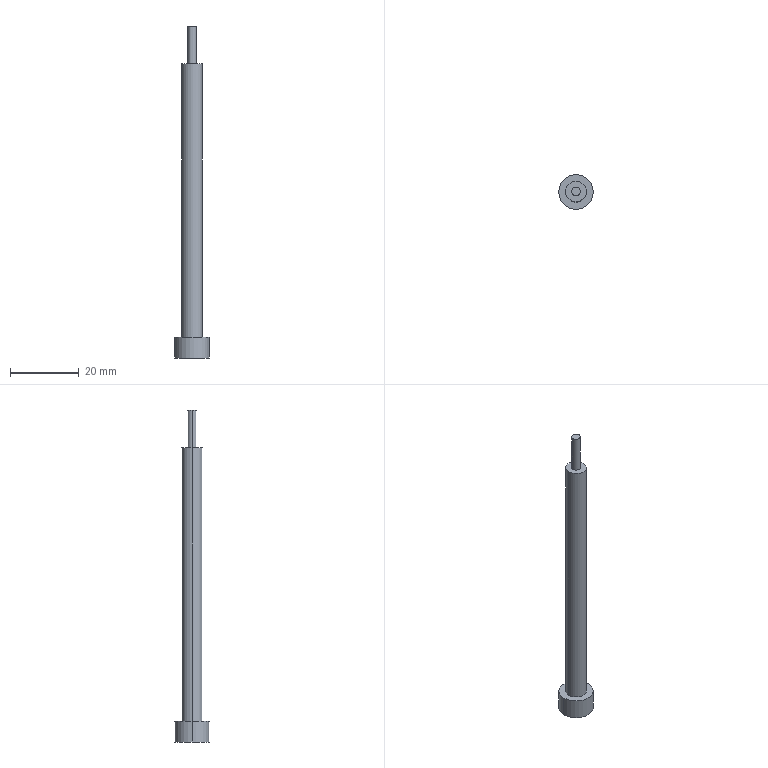Part | Creo | 1 solid | 10 faces | box 10 x 10 x 96.628 mm | volume 2777 mm3 | cylinder 6 | plane 4 | commonest cylinder face diameters 2.5 x2 6 x2 10 x2
STEP:
#1=CARTESIAN_POINT('',(-84.,-40.5,-87.5));
#2=VERTEX_POINT('',#1);
#3=CARTESIAN_POINT('',(-94.,-40.5,-87.5));
#4=VERTEX_POINT('',#3);
#5=CARTESIAN_POINT('',(-89.,-40.5,-87.5));
#6=DIRECTION('',(0.,0.,1.));
#7=DIRECTION('',(1.,0.,0.));
#8=AXIS2_PLACEMENT_3D('',#5,#6,#7);
#9=CIRCLE('',#8,5.);
#10=EDGE_CURVE('',#2,#4,#9,.T.);
#11=ORIENTED_EDGE('',*,*,#10,.F.);
#12=CARTESIAN_POINT('',(-89.,-40.5,-87.5));
#13=DIRECTION('',(0.,0.,1.));
#14=DIRECTION('',(-1.,0.,0.));
#15=AXIS2_PLACEMENT_3D('',#12,#13,#14);
#16=CIRCLE('',#15,5.);
#17=EDGE_CURVE('',#4,#2,#16,.T.);
#18=ORIENTED_EDGE('',*,*,#17,.F.);
#19=EDGE_LOOP('',(#11,#18));
#20=FACE_OUTER_BOUND('',#19,.F.);
#21=CARTESIAN_POINT('',(-86.,-40.5,-87.5));
#22=VERTEX_POINT('',#21);
#23=CARTESIAN_POINT('',(-92.,-40.5,-87.5));
#24=VERTEX_POINT('',#23);
#25=CARTESIAN_POINT('',(-89.,-40.5,-87.5));
#26=DIRECTION('',(0.,0.,-1.));
#27=DIRECTION('',(1.,0.,0.));
#28=AXIS2_PLACEMENT_3D('',#25,#26,#27);
#29=CIRCLE('',#28,3.);
#30=EDGE_CURVE('',#22,#24,#29,.T.);
#31=ORIENTED_EDGE('',*,*,#30,.F.);
#32=CARTESIAN_POINT('',(-89.,-40.5,-87.5));
#33=DIRECTION('',(0.,0.,-1.));
#34=DIRECTION('',(-1.,0.,0.));
#35=AXIS2_PLACEMENT_3D('',#32,#33,#34);
#36=CIRCLE('',#35,3.);
#37=EDGE_CURVE('',#24,#22,#36,.T.);
#38=ORIENTED_EDGE('',*,*,#37,.F.);
#39=EDGE_LOOP('',(#31,#38));
#40=FACE_BOUND('',#39,.F.);
#41=CARTESIAN_POINT('',(-89.,-40.5,-87.5));
#42=DIRECTION('',(0.,0.,1.));
#43=DIRECTION('',(1.,0.,0.));
#44=AXIS2_PLACEMENT_3D('',#41,#42,#43);
#45=PLANE('',#44);
#46=ADVANCED_FACE('',(#20,#40),#45,.T.);
#47=CARTESIAN_POINT('',(-92.,-40.5,-7.872));
#48=VERTEX_POINT('',#47);
#49=CARTESIAN_POINT('',(-86.,-40.5,-7.872));
#50=VERTEX_POINT('',#49);
#51=CARTESIAN_POINT('',(-89.,-40.5,-7.872));
#52=DIRECTION('',(0.,0.,1.));
#53=DIRECTION('',(-1.,0.,0.));
#54=AXIS2_PLACEMENT_3D('',#51,#52,#53);
#55=CIRCLE('',#54,3.);
#56=EDGE_CURVE('',#48,#50,#55,.T.);
#57=ORIENTED_EDGE('',*,*,#56,.T.);
#58=CARTESIAN_POINT('',(-86.,-40.5,-87.5));
#59=DIRECTION('',(0.,0.,1.));
#60=VECTOR('',#59,79.628);
#61=LINE('',#58,#60);
#62=EDGE_CURVE('',#22,#50,#61,.T.);
#63=ORIENTED_EDGE('',*,*,#62,.F.);
#64=ORIENTED_EDGE('',*,*,#30,.T.);
#65=CARTESIAN_POINT('',(-92.,-40.5,-87.5));
#66=DIRECTION('',(0.,0.,1.));
#67=VECTOR('',#66,79.628);
#68=LINE('',#65,#67);
#69=EDGE_CURVE('',#24,#48,#68,.T.);
#70=ORIENTED_EDGE('',*,*,#69,.T.);
#71=EDGE_LOOP('',(#57,#63,#64,#70));
#72=FACE_OUTER_BOUND('',#71,.F.);
#73=CARTESIAN_POINT('',(-89.,-40.5,-87.5));
#74=DIRECTION('',(0.,0.,1.));
#75=DIRECTION('',(1.,0.,0.));
#76=AXIS2_PLACEMENT_3D('',#73,#74,#75);
#77=CYLINDRICAL_SURFACE('',#76,3.);
#78=ADVANCED_FACE('',(#72),#77,.T.);
#79=ORIENTED_EDGE('',*,*,#56,.F.);
#80=CARTESIAN_POINT('',(-89.,-40.5,-7.872));
#81=DIRECTION('',(0.,0.,1.));
#82=DIRECTION('',(1.,0.,0.));
#83=AXIS2_PLACEMENT_3D('',#80,#81,#82);
#84=CIRCLE('',#83,3.);
#85=EDGE_CURVE('',#50,#48,#84,.T.);
#86=ORIENTED_EDGE('',*,*,#85,.F.);
#87=EDGE_LOOP('',(#79,#86));
#88=FACE_OUTER_BOUND('',#87,.F.);
#89=CARTESIAN_POINT('',(-90.25,-40.5,-7.872));
#90=VERTEX_POINT('',#89);
#91=CARTESIAN_POINT('',(-87.75,-40.5,-7.872));
#92=VERTEX_POINT('',#91);
#93=CARTESIAN_POINT('',(-89.,-40.5,-7.872));
#94=DIRECTION('',(0.,0.,-1.));
#95=DIRECTION('',(-1.,0.,0.));
#96=AXIS2_PLACEMENT_3D('',#93,#94,#95);
#97=CIRCLE('',#96,1.25);
#98=EDGE_CURVE('',#90,#92,#97,.T.);
#99=ORIENTED_EDGE('',*,*,#98,.F.);
#100=CARTESIAN_POINT('',(-89.,-40.5,-7.872));
#101=DIRECTION('',(0.,0.,-1.));
#102=DIRECTION('',(1.,0.,0.));
#103=AXIS2_PLACEMENT_3D('',#100,#101,#102);
#104=CIRCLE('',#103,1.25);
#105=EDGE_CURVE('',#92,#90,#104,.T.);
#106=ORIENTED_EDGE('',*,*,#105,.F.);
#107=EDGE_LOOP('',(#99,#106));
#108=FACE_BOUND('',#107,.F.);
#109=CARTESIAN_POINT('',(-89.,-40.5,-7.872));
#110=DIRECTION('',(0.,0.,-1.));
#111=DIRECTION('',(0.,1.,0.));
#112=AXIS2_PLACEMENT_3D('',#109,#110,#111);
#113=PLANE('',#112);
#114=ADVANCED_FACE('',(#88,#108),#113,.F.);
#115=CARTESIAN_POINT('',(-87.75,-40.5,3.128));
#116=VERTEX_POINT('',#115);
#117=CARTESIAN_POINT('',(-90.25,-40.5,3.128));
#118=VERTEX_POINT('',#117);
#119=CARTESIAN_POINT('',(-89.,-40.5,3.128));
#120=DIRECTION('',(0.,0.,1.));
#121=DIRECTION('',(1.,0.,0.));
#122=AXIS2_PLACEMENT_3D('',#119,#120,#121);
#123=CIRCLE('',#122,1.25);
#124=EDGE_CURVE('',#116,#118,#123,.T.);
#125=ORIENTED_EDGE('',*,*,#124,.T.);
#126=CARTESIAN_POINT('',(-90.25,-40.5,-7.872));
#127=DIRECTION('',(0.,0.,1.));
#128=VECTOR('',#127,11.);
#129=LINE('',#126,#128);
#130=EDGE_CURVE('',#90,#118,#129,.T.);
#131=ORIENTED_EDGE('',*,*,#130,.F.);
#132=ORIENTED_EDGE('',*,*,#98,.T.);
#133=CARTESIAN_POINT('',(-87.75,-40.5,-7.872));
#134=DIRECTION('',(0.,0.,1.));
#135=VECTOR('',#134,11.);
#136=LINE('',#133,#135);
#137=EDGE_CURVE('',#92,#116,#136,.T.);
#138=ORIENTED_EDGE('',*,*,#137,.T.);
#139=EDGE_LOOP('',(#125,#131,#132,#138));
#140=FACE_OUTER_BOUND('',#139,.F.);
#141=CARTESIAN_POINT('',(-89.,-40.5,-6.872));
#142=DIRECTION('',(0.,0.,1.));
#143=DIRECTION('',(1.,0.,0.));
#144=AXIS2_PLACEMENT_3D('',#141,#142,#143);
#145=CYLINDRICAL_SURFACE('',#144,1.25);
#146=ADVANCED_FACE('',(#140),#145,.T.);
#147=ORIENTED_EDGE('',*,*,#124,.F.);
#148=CARTESIAN_POINT('',(-89.,-40.5,3.128));
#149=DIRECTION('',(0.,0.,1.));
#150=DIRECTION('',(-1.,0.,0.));
#151=AXIS2_PLACEMENT_3D('',#148,#149,#150);
#152=CIRCLE('',#151,1.25);
#153=EDGE_CURVE('',#118,#116,#152,.T.);
#154=ORIENTED_EDGE('',*,*,#153,.F.);
#155=EDGE_LOOP('',(#147,#154));
#156=FACE_OUTER_BOUND('',#155,.F.);
#157=CARTESIAN_POINT('',(0.,0.,3.128));
#158=DIRECTION('',(0.,0.,1.));
#159=DIRECTION('',(0.,1.,0.));
#160=AXIS2_PLACEMENT_3D('',#157,#158,#159);
#161=PLANE('',#160);
#162=ADVANCED_FACE('',(#156),#161,.T.);
#163=ORIENTED_EDGE('',*,*,#153,.T.);
#164=ORIENTED_EDGE('',*,*,#137,.F.);
#165=ORIENTED_EDGE('',*,*,#105,.T.);
#166=ORIENTED_EDGE('',*,*,#130,.T.);
#167=EDGE_LOOP('',(#163,#164,#165,#166));
#168=FACE_OUTER_BOUND('',#167,.F.);
#169=CARTESIAN_POINT('',(-89.,-40.5,-6.872));
#170=DIRECTION('',(0.,0.,1.));
#171=DIRECTION('',(1.,0.,0.));
#172=AXIS2_PLACEMENT_3D('',#169,#170,#171);
#173=CYLINDRICAL_SURFACE('',#172,1.25);
#174=ADVANCED_FACE('',(#168),#173,.T.);
#175=ORIENTED_EDGE('',*,*,#85,.T.);
#176=ORIENTED_EDGE('',*,*,#69,.F.);
#177=ORIENTED_EDGE('',*,*,#37,.T.);
#178=ORIENTED_EDGE('',*,*,#62,.T.);
#179=EDGE_LOOP('',(#175,#176,#177,#178));
#180=FACE_OUTER_BOUND('',#179,.F.);
#181=CARTESIAN_POINT('',(-89.,-40.5,-87.5));
#182=DIRECTION('',(0.,0.,1.));
#183=DIRECTION('',(1.,0.,0.));
#184=AXIS2_PLACEMENT_3D('',#181,#182,#183);
#185=CYLINDRICAL_SURFACE('',#184,3.);
#186=ADVANCED_FACE('',(#180),#185,.T.);
#187=ORIENTED_EDGE('',*,*,#10,.T.);
#188=CARTESIAN_POINT('',(-94.,-40.5,-93.5));
#189=VERTEX_POINT('',#188);
#190=CARTESIAN_POINT('',(-94.,-40.5,-93.5));
#191=DIRECTION('',(0.,0.,1.));
#192=VECTOR('',#191,6.);
#193=LINE('',#190,#192);
#194=EDGE_CURVE('',#189,#4,#193,.T.);
#195=ORIENTED_EDGE('',*,*,#194,.F.);
#196=CARTESIAN_POINT('',(-84.,-40.5,-93.5));
#197=VERTEX_POINT('',#196);
#198=CARTESIAN_POINT('',(-89.,-40.5,-93.5));
#199=DIRECTION('',(0.,0.,-1.));
#200=DIRECTION('',(-1.,0.,0.));
#201=AXIS2_PLACEMENT_3D('',#198,#199,#200);
#202=CIRCLE('',#201,5.);
#203=EDGE_CURVE('',#189,#197,#202,.T.);
#204=ORIENTED_EDGE('',*,*,#203,.T.);
#205=CARTESIAN_POINT('',(-84.,-40.5,-93.5));
#206=DIRECTION('',(0.,0.,1.));
#207=VECTOR('',#206,6.);
#208=LINE('',#205,#207);
#209=EDGE_CURVE('',#197,#2,#208,.T.);
#210=ORIENTED_EDGE('',*,*,#209,.T.);
#211=EDGE_LOOP('',(#187,#195,#204,#210));
#212=FACE_OUTER_BOUND('',#211,.F.);
#213=CARTESIAN_POINT('',(-89.,-40.5,-93.5));
#214=DIRECTION('',(0.,0.,1.));
#215=DIRECTION('',(1.,0.,0.));
#216=AXIS2_PLACEMENT_3D('',#213,#214,#215);
#217=CYLINDRICAL_SURFACE('',#216,5.);
#218=ADVANCED_FACE('',(#212),#217,.T.);
#219=ORIENTED_EDGE('',*,*,#17,.T.);
#220=ORIENTED_EDGE('',*,*,#209,.F.);
#221=CARTESIAN_POINT('',(-89.,-40.5,-93.5));
#222=DIRECTION('',(0.,0.,-1.));
#223=DIRECTION('',(1.,0.,0.));
#224=AXIS2_PLACEMENT_3D('',#221,#222,#223);
#225=CIRCLE('',#224,5.);
#226=EDGE_CURVE('',#197,#189,#225,.T.);
#227=ORIENTED_EDGE('',*,*,#226,.T.);
#228=ORIENTED_EDGE('',*,*,#194,.T.);
#229=EDGE_LOOP('',(#219,#220,#227,#228));
#230=FACE_OUTER_BOUND('',#229,.F.);
#231=CARTESIAN_POINT('',(-89.,-40.5,-93.5));
#232=DIRECTION('',(0.,0.,1.));
#233=DIRECTION('',(1.,0.,0.));
#234=AXIS2_PLACEMENT_3D('',#231,#232,#233);
#235=CYLINDRICAL_SURFACE('',#234,5.);
#236=ADVANCED_FACE('',(#230),#235,.T.);
#237=ORIENTED_EDGE('',*,*,#203,.F.);
#238=ORIENTED_EDGE('',*,*,#226,.F.);
#239=EDGE_LOOP('',(#237,#238));
#240=FACE_OUTER_BOUND('',#239,.F.);
#241=CARTESIAN_POINT('',(-89.,-40.5,-93.5));
#242=DIRECTION('',(0.,0.,-1.));
#243=DIRECTION('',(-1.,0.,0.));
#244=AXIS2_PLACEMENT_3D('',#241,#242,#243);
#245=PLANE('',#244);
#246=ADVANCED_FACE('',(#240),#245,.T.);
#247=CLOSED_SHELL('',(#46,#78,#114,#146,#162,#174,#186,#218,#236,#246));
#248=MANIFOLD_SOLID_BREP('',#247);
#249=(LENGTH_UNIT()NAMED_UNIT(*)SI_UNIT(.MILLI.,.METRE.));
#250=UNCERTAINTY_MEASURE_WITH_UNIT(LENGTH_MEASURE(0.009765),#249,'','');
#251=(NAMED_UNIT(*)PLANE_ANGLE_UNIT()SI_UNIT($,.RADIAN.));
#252=PLANE_ANGLE_MEASURE_WITH_UNIT(PLANE_ANGLE_MEASURE(0.01745),#251);
#253=(CONVERSION_BASED_UNIT('DEGREE',#252)NAMED_UNIT(*)PLANE_ANGLE_UNIT());
#254=(NAMED_UNIT(*)SI_UNIT($,.STERADIAN.)SOLID_ANGLE_UNIT());
#255=(GEOMETRIC_REPRESENTATION_CONTEXT(3)GLOBAL_UNCERTAINTY_ASSIGNED_CONTEXT((#250))GLOBAL_UNIT_ASSIGNED_CONTEXT((#249,#253,#254))REPRESENTATION_CONTEXT('',''));
#256=ADVANCED_BREP_SHAPE_REPRESENTATION('',(#248),#255);